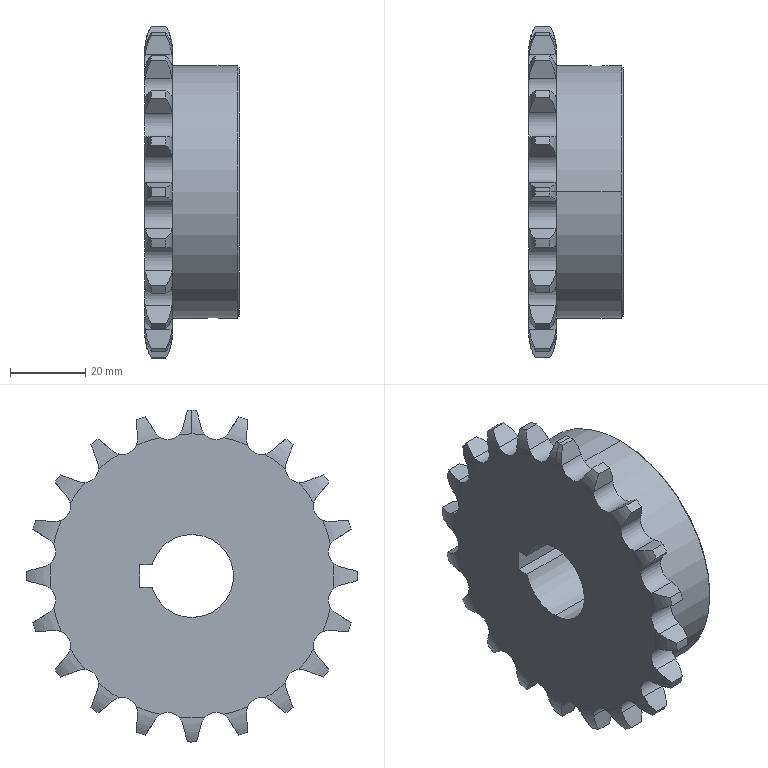Part | STEP file | RS40-1B20T-SS-H22_with key | 1 solid | 141 faces | box 25 x 88 x 88 mm | volume 86661 mm3 | cylinder 50 | plane 47 | torus 42 | cone 2 | commonest cylinder face diameters 88 x21 7.92 x20 6 x4 22 x3 67 x2